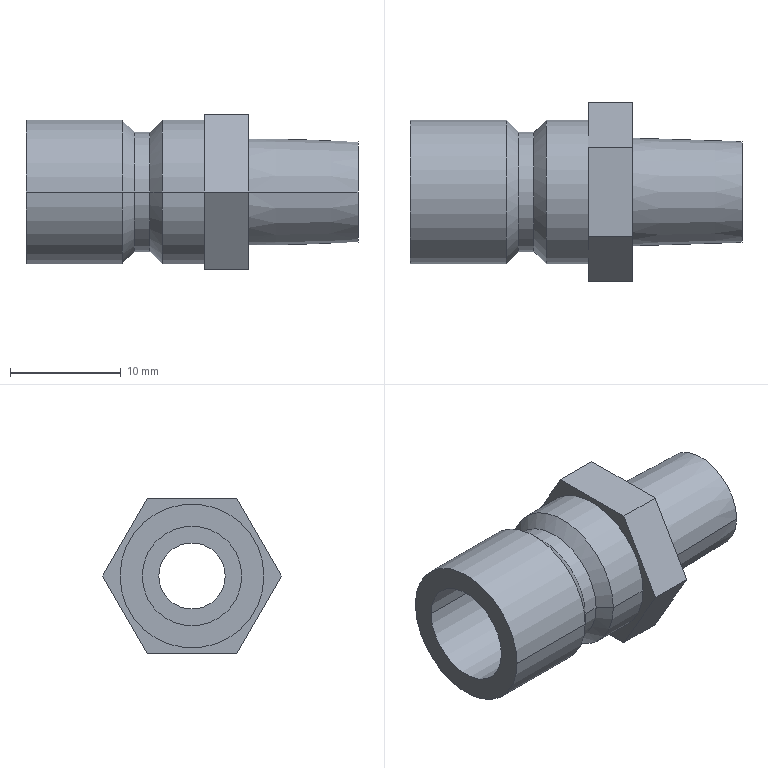Part | Creo | 1 solid | 27 faces | box 30 x 16.166 x 14 mm | volume 1882 mm3 | plane 11 | cylinder 10 | cone 6 | commonest cylinder face diameters 13 x4 6 x2 9 x2 10.8 x2
STEP:
#1=CARTESIAN_POINT('',(0.,0.,0.));
#2=DIRECTION('',(0.,0.,1.));
#3=DIRECTION('',(1.,0.,0.));
#4=AXIS2_PLACEMENT_3D('',#1,#2,#3);
#5=CARTESIAN_POINT('',(-220.1,-3.5,-74.09));
#6=VERTEX_POINT('',#5);
#7=CARTESIAN_POINT('',(-220.1,-16.5,-74.09));
#8=VERTEX_POINT('',#7);
#9=CARTESIAN_POINT('',(-220.1,-10.,-74.09));
#10=DIRECTION('',(-1.,0.,0.));
#11=DIRECTION('',(0.,1.,0.));
#12=AXIS2_PLACEMENT_3D('',#9,#10,#11);
#13=CIRCLE('',#12,6.5);
#14=EDGE_CURVE('',#6,#8,#13,.T.);
#15=ORIENTED_EDGE('',*,*,#14,.F.);
#16=CARTESIAN_POINT('',(-220.1,-10.,-74.09));
#17=DIRECTION('',(-1.,0.,0.));
#18=DIRECTION('',(0.,-1.,0.));
#19=AXIS2_PLACEMENT_3D('',#16,#17,#18);
#20=CIRCLE('',#19,6.5);
#21=EDGE_CURVE('',#8,#6,#20,.T.);
#22=ORIENTED_EDGE('',*,*,#21,.F.);
#23=EDGE_LOOP('',(#15,#22));
#24=FACE_OUTER_BOUND('',#23,.F.);
#25=CARTESIAN_POINT('',(-220.1,-5.5,-74.09));
#26=VERTEX_POINT('',#25);
#27=CARTESIAN_POINT('',(-220.1,-14.5,-74.09));
#28=VERTEX_POINT('',#27);
#29=CARTESIAN_POINT('',(-220.1,-10.,-74.09));
#30=DIRECTION('',(1.,0.,0.));
#31=DIRECTION('',(0.,1.,0.));
#32=AXIS2_PLACEMENT_3D('',#29,#30,#31);
#33=CIRCLE('',#32,4.5);
#34=EDGE_CURVE('',#26,#28,#33,.T.);
#35=ORIENTED_EDGE('',*,*,#34,.F.);
#36=CARTESIAN_POINT('',(-220.1,-10.,-74.09));
#37=DIRECTION('',(1.,0.,0.));
#38=DIRECTION('',(0.,-1.,0.));
#39=AXIS2_PLACEMENT_3D('',#36,#37,#38);
#40=CIRCLE('',#39,4.5);
#41=EDGE_CURVE('',#28,#26,#40,.T.);
#42=ORIENTED_EDGE('',*,*,#41,.F.);
#43=EDGE_LOOP('',(#35,#42));
#44=FACE_BOUND('',#43,.F.);
#45=CARTESIAN_POINT('',(-220.1,-10.,-67.59));
#46=DIRECTION('',(-1.,0.,0.));
#47=DIRECTION('',(0.,-1.,0.));
#48=AXIS2_PLACEMENT_3D('',#45,#46,#47);
#49=PLANE('',#48);
#50=ADVANCED_FACE('',(#24,#44),#49,.T.);
#51=ORIENTED_EDGE('',*,*,#14,.T.);
#52=CARTESIAN_POINT('',(-211.4,-16.5,-74.09));
#53=VERTEX_POINT('',#52);
#54=CARTESIAN_POINT('',(-220.1,-16.5,-74.09));
#55=DIRECTION('',(1.,0.,0.));
#56=VECTOR('',#55,8.7);
#57=LINE('',#54,#56);
#58=EDGE_CURVE('',#8,#53,#57,.T.);
#59=ORIENTED_EDGE('',*,*,#58,.T.);
#60=CARTESIAN_POINT('',(-211.4,-3.5,-74.09));
#61=VERTEX_POINT('',#60);
#62=CARTESIAN_POINT('',(-211.4,-10.,-74.09));
#63=DIRECTION('',(1.,0.,0.));
#64=DIRECTION('',(0.,-1.,0.));
#65=AXIS2_PLACEMENT_3D('',#62,#63,#64);
#66=CIRCLE('',#65,6.5);
#67=EDGE_CURVE('',#53,#61,#66,.T.);
#68=ORIENTED_EDGE('',*,*,#67,.T.);
#69=CARTESIAN_POINT('',(-220.1,-3.5,-74.09));
#70=DIRECTION('',(1.,0.,0.));
#71=VECTOR('',#70,8.7);
#72=LINE('',#69,#71);
#73=EDGE_CURVE('',#6,#61,#72,.T.);
#74=ORIENTED_EDGE('',*,*,#73,.F.);
#75=EDGE_LOOP('',(#51,#59,#68,#74));
#76=FACE_OUTER_BOUND('',#75,.F.);
#77=CARTESIAN_POINT('',(-200.,-10.,-74.09));
#78=DIRECTION('',(1.,0.,0.));
#79=DIRECTION('',(0.,1.,0.));
#80=AXIS2_PLACEMENT_3D('',#77,#78,#79);
#81=CYLINDRICAL_SURFACE('',#80,6.5);
#82=ADVANCED_FACE('',(#76),#81,.T.);
#83=ORIENTED_EDGE('',*,*,#21,.T.);
#84=ORIENTED_EDGE('',*,*,#73,.T.);
#85=CARTESIAN_POINT('',(-211.4,-10.,-74.09));
#86=DIRECTION('',(1.,0.,0.));
#87=DIRECTION('',(0.,1.,0.));
#88=AXIS2_PLACEMENT_3D('',#85,#86,#87);
#89=CIRCLE('',#88,6.5);
#90=EDGE_CURVE('',#61,#53,#89,.T.);
#91=ORIENTED_EDGE('',*,*,#90,.T.);
#92=ORIENTED_EDGE('',*,*,#58,.F.);
#93=EDGE_LOOP('',(#83,#84,#91,#92));
#94=FACE_OUTER_BOUND('',#93,.F.);
#95=CARTESIAN_POINT('',(-200.,-10.,-74.09));
#96=DIRECTION('',(1.,0.,0.));
#97=DIRECTION('',(0.,1.,0.));
#98=AXIS2_PLACEMENT_3D('',#95,#96,#97);
#99=CYLINDRICAL_SURFACE('',#98,6.5);
#100=ADVANCED_FACE('',(#94),#99,.T.);
#101=ORIENTED_EDGE('',*,*,#90,.F.);
#102=CARTESIAN_POINT('',(-210.3,-4.6,-74.09));
#103=VERTEX_POINT('',#102);
#104=CARTESIAN_POINT('',(-210.3,-4.6,-74.09));
#105=DIRECTION('',(-0.7071,0.7071,0.));
#106=VECTOR('',#105,1.556);
#107=LINE('',#104,#106);
#108=EDGE_CURVE('',#103,#61,#107,.T.);
#109=ORIENTED_EDGE('',*,*,#108,.F.);
#110=CARTESIAN_POINT('',(-210.3,-15.4,-74.09));
#111=VERTEX_POINT('',#110);
#112=CARTESIAN_POINT('',(-210.3,-10.,-74.09));
#113=DIRECTION('',(-1.,0.,0.));
#114=DIRECTION('',(0.,-1.,0.));
#115=AXIS2_PLACEMENT_3D('',#112,#113,#114);
#116=CIRCLE('',#115,5.4);
#117=EDGE_CURVE('',#111,#103,#116,.T.);
#118=ORIENTED_EDGE('',*,*,#117,.F.);
#119=CARTESIAN_POINT('',(-210.3,-15.4,-74.09));
#120=DIRECTION('',(-0.7071,-0.7071,0.));
#121=VECTOR('',#120,1.556);
#122=LINE('',#119,#121);
#123=EDGE_CURVE('',#111,#53,#122,.T.);
#124=ORIENTED_EDGE('',*,*,#123,.T.);
#125=EDGE_LOOP('',(#101,#109,#118,#124));
#126=FACE_OUTER_BOUND('',#125,.F.);
#127=CARTESIAN_POINT('',(-210.85,-10.,-74.09));
#128=DIRECTION('',(-1.,0.,0.));
#129=DIRECTION('',(0.,-1.,0.));
#130=AXIS2_PLACEMENT_3D('',#127,#128,#129);
#131=CONICAL_SURFACE('',#130,5.95,45.);
#132=ADVANCED_FACE('',(#126),#131,.T.);
#133=ORIENTED_EDGE('',*,*,#67,.F.);
#134=ORIENTED_EDGE('',*,*,#123,.F.);
#135=CARTESIAN_POINT('',(-210.3,-10.,-74.09));
#136=DIRECTION('',(-1.,0.,0.));
#137=DIRECTION('',(0.,1.,0.));
#138=AXIS2_PLACEMENT_3D('',#135,#136,#137);
#139=CIRCLE('',#138,5.4);
#140=EDGE_CURVE('',#103,#111,#139,.T.);
#141=ORIENTED_EDGE('',*,*,#140,.F.);
#142=ORIENTED_EDGE('',*,*,#108,.T.);
#143=EDGE_LOOP('',(#133,#134,#141,#142));
#144=FACE_OUTER_BOUND('',#143,.F.);
#145=CARTESIAN_POINT('',(-210.85,-10.,-74.09));
#146=DIRECTION('',(-1.,0.,0.));
#147=DIRECTION('',(0.,-1.,0.));
#148=AXIS2_PLACEMENT_3D('',#145,#146,#147);
#149=CONICAL_SURFACE('',#148,5.95,45.);
#150=ADVANCED_FACE('',(#144),#149,.T.);
#151=ORIENTED_EDGE('',*,*,#140,.T.);
#152=CARTESIAN_POINT('',(-208.9,-15.4,-74.09));
#153=VERTEX_POINT('',#152);
#154=CARTESIAN_POINT('',(-210.3,-15.4,-74.09));
#155=DIRECTION('',(1.,0.,0.));
#156=VECTOR('',#155,1.4);
#157=LINE('',#154,#156);
#158=EDGE_CURVE('',#111,#153,#157,.T.);
#159=ORIENTED_EDGE('',*,*,#158,.T.);
#160=CARTESIAN_POINT('',(-208.9,-4.6,-74.09));
#161=VERTEX_POINT('',#160);
#162=CARTESIAN_POINT('',(-208.9,-10.,-74.09));
#163=DIRECTION('',(1.,0.,0.));
#164=DIRECTION('',(0.,-1.,0.));
#165=AXIS2_PLACEMENT_3D('',#162,#163,#164);
#166=CIRCLE('',#165,5.4);
#167=EDGE_CURVE('',#153,#161,#166,.T.);
#168=ORIENTED_EDGE('',*,*,#167,.T.);
#169=CARTESIAN_POINT('',(-210.3,-4.6,-74.09));
#170=DIRECTION('',(1.,0.,0.));
#171=VECTOR('',#170,1.4);
#172=LINE('',#169,#171);
#173=EDGE_CURVE('',#103,#161,#172,.T.);
#174=ORIENTED_EDGE('',*,*,#173,.F.);
#175=EDGE_LOOP('',(#151,#159,#168,#174));
#176=FACE_OUTER_BOUND('',#175,.F.);
#177=CARTESIAN_POINT('',(-200.,-10.,-74.09));
#178=DIRECTION('',(1.,0.,0.));
#179=DIRECTION('',(0.,1.,0.));
#180=AXIS2_PLACEMENT_3D('',#177,#178,#179);
#181=CYLINDRICAL_SURFACE('',#180,5.4);
#182=ADVANCED_FACE('',(#176),#181,.T.);
#183=ORIENTED_EDGE('',*,*,#117,.T.);
#184=ORIENTED_EDGE('',*,*,#173,.T.);
#185=CARTESIAN_POINT('',(-208.9,-10.,-74.09));
#186=DIRECTION('',(1.,0.,0.));
#187=DIRECTION('',(0.,1.,0.));
#188=AXIS2_PLACEMENT_3D('',#185,#186,#187);
#189=CIRCLE('',#188,5.4);
#190=EDGE_CURVE('',#161,#153,#189,.T.);
#191=ORIENTED_EDGE('',*,*,#190,.T.);
#192=ORIENTED_EDGE('',*,*,#158,.F.);
#193=EDGE_LOOP('',(#183,#184,#191,#192));
#194=FACE_OUTER_BOUND('',#193,.F.);
#195=CARTESIAN_POINT('',(-200.,-10.,-74.09));
#196=DIRECTION('',(1.,0.,0.));
#197=DIRECTION('',(0.,1.,0.));
#198=AXIS2_PLACEMENT_3D('',#195,#196,#197);
#199=CYLINDRICAL_SURFACE('',#198,5.4);
#200=ADVANCED_FACE('',(#194),#199,.T.);
#201=ORIENTED_EDGE('',*,*,#190,.F.);
#202=CARTESIAN_POINT('',(-207.8,-3.5,-74.09));
#203=VERTEX_POINT('',#202);
#204=CARTESIAN_POINT('',(-208.9,-4.6,-74.09));
#205=DIRECTION('',(0.7071,0.7071,0.));
#206=VECTOR('',#205,1.556);
#207=LINE('',#204,#206);
#208=EDGE_CURVE('',#161,#203,#207,.T.);
#209=ORIENTED_EDGE('',*,*,#208,.T.);
#210=CARTESIAN_POINT('',(-207.8,-16.5,-74.09));
#211=VERTEX_POINT('',#210);
#212=CARTESIAN_POINT('',(-207.8,-10.,-74.09));
#213=DIRECTION('',(-1.,0.,0.));
#214=DIRECTION('',(0.,-1.,0.));
#215=AXIS2_PLACEMENT_3D('',#212,#213,#214);
#216=CIRCLE('',#215,6.5);
#217=EDGE_CURVE('',#211,#203,#216,.T.);
#218=ORIENTED_EDGE('',*,*,#217,.F.);
#219=CARTESIAN_POINT('',(-208.9,-15.4,-74.09));
#220=DIRECTION('',(0.7071,-0.7071,0.));
#221=VECTOR('',#220,1.556);
#222=LINE('',#219,#221);
#223=EDGE_CURVE('',#153,#211,#222,.T.);
#224=ORIENTED_EDGE('',*,*,#223,.F.);
#225=EDGE_LOOP('',(#201,#209,#218,#224));
#226=FACE_OUTER_BOUND('',#225,.F.);
#227=CARTESIAN_POINT('',(-208.35,-10.,-74.09));
#228=DIRECTION('',(1.,0.,0.));
#229=DIRECTION('',(0.,1.,0.));
#230=AXIS2_PLACEMENT_3D('',#227,#228,#229);
#231=CONICAL_SURFACE('',#230,5.95,45.);
#232=ADVANCED_FACE('',(#226),#231,.T.);
#233=ORIENTED_EDGE('',*,*,#167,.F.);
#234=ORIENTED_EDGE('',*,*,#223,.T.);
#235=CARTESIAN_POINT('',(-207.8,-10.,-74.09));
#236=DIRECTION('',(-1.,0.,0.));
#237=DIRECTION('',(0.,1.,0.));
#238=AXIS2_PLACEMENT_3D('',#235,#236,#237);
#239=CIRCLE('',#238,6.5);
#240=EDGE_CURVE('',#203,#211,#239,.T.);
#241=ORIENTED_EDGE('',*,*,#240,.F.);
#242=ORIENTED_EDGE('',*,*,#208,.F.);
#243=EDGE_LOOP('',(#233,#234,#241,#242));
#244=FACE_OUTER_BOUND('',#243,.F.);
#245=CARTESIAN_POINT('',(-208.35,-10.,-74.09));
#246=DIRECTION('',(1.,0.,0.));
#247=DIRECTION('',(0.,1.,0.));
#248=AXIS2_PLACEMENT_3D('',#245,#246,#247);
#249=CONICAL_SURFACE('',#248,5.95,45.);
#250=ADVANCED_FACE('',(#244),#249,.T.);
#251=ORIENTED_EDGE('',*,*,#240,.T.);
#252=CARTESIAN_POINT('',(-204.,-16.5,-74.09));
#253=VERTEX_POINT('',#252);
#254=CARTESIAN_POINT('',(-207.8,-16.5,-74.09));
#255=DIRECTION('',(1.,0.,0.));
#256=VECTOR('',#255,3.8);
#257=LINE('',#254,#256);
#258=EDGE_CURVE('',#211,#253,#257,.T.);
#259=ORIENTED_EDGE('',*,*,#258,.T.);
#260=CARTESIAN_POINT('',(-204.,-3.5,-74.09));
#261=VERTEX_POINT('',#260);
#262=CARTESIAN_POINT('',(-204.,-10.,-74.09));
#263=DIRECTION('',(1.,0.,0.));
#264=DIRECTION('',(0.,-1.,0.));
#265=AXIS2_PLACEMENT_3D('',#262,#263,#264);
#266=CIRCLE('',#265,6.5);
#267=EDGE_CURVE('',#253,#261,#266,.T.);
#268=ORIENTED_EDGE('',*,*,#267,.T.);
#269=CARTESIAN_POINT('',(-207.8,-3.5,-74.09));
#270=DIRECTION('',(1.,0.,0.));
#271=VECTOR('',#270,3.8);
#272=LINE('',#269,#271);
#273=EDGE_CURVE('',#203,#261,#272,.T.);
#274=ORIENTED_EDGE('',*,*,#273,.F.);
#275=EDGE_LOOP('',(#251,#259,#268,#274));
#276=FACE_OUTER_BOUND('',#275,.F.);
#277=CARTESIAN_POINT('',(-200.,-10.,-74.09));
#278=DIRECTION('',(1.,0.,0.));
#279=DIRECTION('',(0.,1.,0.));
#280=AXIS2_PLACEMENT_3D('',#277,#278,#279);
#281=CYLINDRICAL_SURFACE('',#280,6.5);
#282=ADVANCED_FACE('',(#276),#281,.T.);
#283=ORIENTED_EDGE('',*,*,#217,.T.);
#284=ORIENTED_EDGE('',*,*,#273,.T.);
#285=CARTESIAN_POINT('',(-204.,-10.,-74.09));
#286=DIRECTION('',(1.,0.,0.));
#287=DIRECTION('',(0.,1.,0.));
#288=AXIS2_PLACEMENT_3D('',#285,#286,#287);
#289=CIRCLE('',#288,6.5);
#290=EDGE_CURVE('',#261,#253,#289,.T.);
#291=ORIENTED_EDGE('',*,*,#290,.T.);
#292=ORIENTED_EDGE('',*,*,#258,.F.);
#293=EDGE_LOOP('',(#283,#284,#291,#292));
#294=FACE_OUTER_BOUND('',#293,.F.);
#295=CARTESIAN_POINT('',(-200.,-10.,-74.09));
#296=DIRECTION('',(1.,0.,0.));
#297=DIRECTION('',(0.,1.,0.));
#298=AXIS2_PLACEMENT_3D('',#295,#296,#297);
#299=CYLINDRICAL_SURFACE('',#298,6.5);
#300=ADVANCED_FACE('',(#294),#299,.T.);
#301=CARTESIAN_POINT('',(-204.,-18.083,-74.09));
#302=VERTEX_POINT('',#301);
#303=CARTESIAN_POINT('',(-204.,-14.041,-67.09));
#304=VERTEX_POINT('',#303);
#305=CARTESIAN_POINT('',(-204.,-18.083,-74.09));
#306=DIRECTION('',(0.,0.5,0.866));
#307=VECTOR('',#306,8.083);
#308=LINE('',#305,#307);
#309=EDGE_CURVE('',#302,#304,#308,.T.);
#310=ORIENTED_EDGE('',*,*,#309,.F.);
#311=CARTESIAN_POINT('',(-204.,-14.041,-81.09));
#312=VERTEX_POINT('',#311);
#313=CARTESIAN_POINT('',(-204.,-14.041,-81.09));
#314=DIRECTION('',(0.,-0.5,0.866));
#315=VECTOR('',#314,8.083);
#316=LINE('',#313,#315);
#317=EDGE_CURVE('',#312,#302,#316,.T.);
#318=ORIENTED_EDGE('',*,*,#317,.F.);
#319=CARTESIAN_POINT('',(-204.,-5.959,-81.09));
#320=VERTEX_POINT('',#319);
#321=CARTESIAN_POINT('',(-204.,-5.959,-81.09));
#322=DIRECTION('',(0.,-1.,0.));
#323=VECTOR('',#322,8.083);
#324=LINE('',#321,#323);
#325=EDGE_CURVE('',#320,#312,#324,.T.);
#326=ORIENTED_EDGE('',*,*,#325,.F.);
#327=CARTESIAN_POINT('',(-204.,-1.917,-74.09));
#328=VERTEX_POINT('',#327);
#329=CARTESIAN_POINT('',(-204.,-1.917,-74.09));
#330=DIRECTION('',(0.,-0.5,-0.866));
#331=VECTOR('',#330,8.083);
#332=LINE('',#329,#331);
#333=EDGE_CURVE('',#328,#320,#332,.T.);
#334=ORIENTED_EDGE('',*,*,#333,.F.);
#335=CARTESIAN_POINT('',(-204.,-5.959,-67.09));
#336=VERTEX_POINT('',#335);
#337=CARTESIAN_POINT('',(-204.,-5.959,-67.09));
#338=DIRECTION('',(0.,0.5,-0.866));
#339=VECTOR('',#338,8.083);
#340=LINE('',#337,#339);
#341=EDGE_CURVE('',#336,#328,#340,.T.);
#342=ORIENTED_EDGE('',*,*,#341,.F.);
#343=CARTESIAN_POINT('',(-204.,-14.041,-67.09));
#344=DIRECTION('',(0.,1.,0.));
#345=VECTOR('',#344,8.083);
#346=LINE('',#343,#345);
#347=EDGE_CURVE('',#304,#336,#346,.T.);
#348=ORIENTED_EDGE('',*,*,#347,.F.);
#349=EDGE_LOOP('',(#310,#318,#326,#334,#342,#348));
#350=FACE_OUTER_BOUND('',#349,.F.);
#351=ORIENTED_EDGE('',*,*,#290,.F.);
#352=ORIENTED_EDGE('',*,*,#267,.F.);
#353=EDGE_LOOP('',(#351,#352));
#354=FACE_BOUND('',#353,.F.);
#355=CARTESIAN_POINT('',(-204.,-10.,-67.09));
#356=DIRECTION('',(-1.,0.,0.));
#357=DIRECTION('',(0.,-1.,0.));
#358=AXIS2_PLACEMENT_3D('',#355,#356,#357);
#359=PLANE('',#358);
#360=ADVANCED_FACE('',(#350,#354),#359,.T.);
#361=ORIENTED_EDGE('',*,*,#309,.T.);
#362=CARTESIAN_POINT('',(-200.,-14.041,-67.09));
#363=VERTEX_POINT('',#362);
#364=CARTESIAN_POINT('',(-200.,-14.041,-67.09));
#365=DIRECTION('',(-1.,0.,0.));
#366=VECTOR('',#365,4.);
#367=LINE('',#364,#366);
#368=EDGE_CURVE('',#363,#304,#367,.T.);
#369=ORIENTED_EDGE('',*,*,#368,.F.);
#370=CARTESIAN_POINT('',(-200.,-18.083,-74.09));
#371=VERTEX_POINT('',#370);
#372=CARTESIAN_POINT('',(-200.,-14.041,-67.09));
#373=DIRECTION('',(0.,-0.5,-0.866));
#374=VECTOR('',#373,8.083);
#375=LINE('',#372,#374);
#376=EDGE_CURVE('',#363,#371,#375,.T.);
#377=ORIENTED_EDGE('',*,*,#376,.T.);
#378=CARTESIAN_POINT('',(-200.,-18.083,-74.09));
#379=DIRECTION('',(-1.,0.,0.));
#380=VECTOR('',#379,4.);
#381=LINE('',#378,#380);
#382=EDGE_CURVE('',#371,#302,#381,.T.);
#383=ORIENTED_EDGE('',*,*,#382,.T.);
#384=EDGE_LOOP('',(#361,#369,#377,#383));
#385=FACE_OUTER_BOUND('',#384,.F.);
#386=CARTESIAN_POINT('',(-204.,-14.041,-67.09));
#387=DIRECTION('',(0.,-0.866,0.5));
#388=DIRECTION('',(0.,0.5,0.866));
#389=AXIS2_PLACEMENT_3D('',#386,#387,#388);
#390=PLANE('',#389);
#391=ADVANCED_FACE('',(#385),#390,.T.);
#392=ORIENTED_EDGE('',*,*,#347,.T.);
#393=CARTESIAN_POINT('',(-200.,-5.959,-67.09));
#394=VERTEX_POINT('',#393);
#395=CARTESIAN_POINT('',(-200.,-5.959,-67.09));
#396=DIRECTION('',(-1.,0.,0.));
#397=VECTOR('',#396,4.);
#398=LINE('',#395,#397);
#399=EDGE_CURVE('',#394,#336,#398,.T.);
#400=ORIENTED_EDGE('',*,*,#399,.F.);
#401=CARTESIAN_POINT('',(-200.,-14.041,-67.09));
#402=DIRECTION('',(0.,1.,0.));
#403=VECTOR('',#402,8.083);
#404=LINE('',#401,#403);
#405=EDGE_CURVE('',#363,#394,#404,.T.);
#406=ORIENTED_EDGE('',*,*,#405,.F.);
#407=ORIENTED_EDGE('',*,*,#368,.T.);
#408=EDGE_LOOP('',(#392,#400,#406,#407));
#409=FACE_OUTER_BOUND('',#408,.F.);
#410=CARTESIAN_POINT('',(-204.,-5.959,-67.09));
#411=DIRECTION('',(0.,0.,1.));
#412=DIRECTION('',(0.,1.,0.));
#413=AXIS2_PLACEMENT_3D('',#410,#411,#412);
#414=PLANE('',#413);
#415=ADVANCED_FACE('',(#409),#414,.T.);
#416=ORIENTED_EDGE('',*,*,#341,.T.);
#417=CARTESIAN_POINT('',(-200.,-1.917,-74.09));
#418=VERTEX_POINT('',#417);
#419=CARTESIAN_POINT('',(-200.,-1.917,-74.09));
#420=DIRECTION('',(-1.,0.,0.));
#421=VECTOR('',#420,4.);
#422=LINE('',#419,#421);
#423=EDGE_CURVE('',#418,#328,#422,.T.);
#424=ORIENTED_EDGE('',*,*,#423,.F.);
#425=CARTESIAN_POINT('',(-200.,-1.917,-74.09));
#426=DIRECTION('',(0.,-0.5,0.866));
#427=VECTOR('',#426,8.083);
#428=LINE('',#425,#427);
#429=EDGE_CURVE('',#418,#394,#428,.T.);
#430=ORIENTED_EDGE('',*,*,#429,.T.);
#431=ORIENTED_EDGE('',*,*,#399,.T.);
#432=EDGE_LOOP('',(#416,#424,#430,#431));
#433=FACE_OUTER_BOUND('',#432,.F.);
#434=CARTESIAN_POINT('',(-204.,-1.917,-74.09));
#435=DIRECTION('',(0.,0.866,0.5));
#436=DIRECTION('',(0.,0.5,-0.866));
#437=AXIS2_PLACEMENT_3D('',#434,#435,#436);
#438=PLANE('',#437);
#439=ADVANCED_FACE('',(#433),#438,.T.);
#440=ORIENTED_EDGE('',*,*,#333,.T.);
#441=CARTESIAN_POINT('',(-200.,-5.959,-81.09));
#442=VERTEX_POINT('',#441);
#443=CARTESIAN_POINT('',(-200.,-5.959,-81.09));
#444=DIRECTION('',(-1.,0.,0.));
#445=VECTOR('',#444,4.);
#446=LINE('',#443,#445);
#447=EDGE_CURVE('',#442,#320,#446,.T.);
#448=ORIENTED_EDGE('',*,*,#447,.F.);
#449=CARTESIAN_POINT('',(-200.,-5.959,-81.09));
#450=DIRECTION('',(0.,0.5,0.866));
#451=VECTOR('',#450,8.083);
#452=LINE('',#449,#451);
#453=EDGE_CURVE('',#442,#418,#452,.T.);
#454=ORIENTED_EDGE('',*,*,#453,.T.);
#455=ORIENTED_EDGE('',*,*,#423,.T.);
#456=EDGE_LOOP('',(#440,#448,#454,#455));
#457=FACE_OUTER_BOUND('',#456,.F.);
#458=CARTESIAN_POINT('',(-204.,-5.959,-81.09));
#459=DIRECTION('',(0.,0.866,-0.5));
#460=DIRECTION('',(0.,-0.5,-0.866));
#461=AXIS2_PLACEMENT_3D('',#458,#459,#460);
#462=PLANE('',#461);
#463=ADVANCED_FACE('',(#457),#462,.T.);
#464=ORIENTED_EDGE('',*,*,#325,.T.);
#465=CARTESIAN_POINT('',(-200.,-14.041,-81.09));
#466=VERTEX_POINT('',#465);
#467=CARTESIAN_POINT('',(-200.,-14.041,-81.09));
#468=DIRECTION('',(-1.,0.,0.));
#469=VECTOR('',#468,4.);
#470=LINE('',#467,#469);
#471=EDGE_CURVE('',#466,#312,#470,.T.);
#472=ORIENTED_EDGE('',*,*,#471,.F.);
#473=CARTESIAN_POINT('',(-200.,-5.959,-81.09));
#474=DIRECTION('',(0.,-1.,0.));
#475=VECTOR('',#474,8.083);
#476=LINE('',#473,#475);
#477=EDGE_CURVE('',#442,#466,#476,.T.);
#478=ORIENTED_EDGE('',*,*,#477,.F.);
#479=ORIENTED_EDGE('',*,*,#447,.T.);
#480=EDGE_LOOP('',(#464,#472,#478,#479));
#481=FACE_OUTER_BOUND('',#480,.F.);
#482=CARTESIAN_POINT('',(-204.,-14.041,-81.09));
#483=DIRECTION('',(0.,0.,-1.));
#484=DIRECTION('',(0.,-1.,0.));
#485=AXIS2_PLACEMENT_3D('',#482,#483,#484);
#486=PLANE('',#485);
#487=ADVANCED_FACE('',(#481),#486,.T.);
#488=ORIENTED_EDGE('',*,*,#317,.T.);
#489=ORIENTED_EDGE('',*,*,#382,.F.);
#490=CARTESIAN_POINT('',(-200.,-18.083,-74.09));
#491=DIRECTION('',(0.,0.5,-0.866));
#492=VECTOR('',#491,8.083);
#493=LINE('',#490,#492);
#494=EDGE_CURVE('',#371,#466,#493,.T.);
#495=ORIENTED_EDGE('',*,*,#494,.T.);
#496=ORIENTED_EDGE('',*,*,#471,.T.);
#497=EDGE_LOOP('',(#488,#489,#495,#496));
#498=FACE_OUTER_BOUND('',#497,.F.);
#499=CARTESIAN_POINT('',(-204.,-18.083,-74.09));
#500=DIRECTION('',(0.,-0.866,-0.5));
#501=DIRECTION('',(0.,-0.5,0.866));
#502=AXIS2_PLACEMENT_3D('',#499,#500,#501);
#503=PLANE('',#502);
#504=ADVANCED_FACE('',(#498),#503,.T.);
#505=ORIENTED_EDGE('',*,*,#453,.F.);
#506=ORIENTED_EDGE('',*,*,#477,.T.);
#507=ORIENTED_EDGE('',*,*,#494,.F.);
#508=ORIENTED_EDGE('',*,*,#376,.F.);
#509=ORIENTED_EDGE('',*,*,#405,.T.);
#510=ORIENTED_EDGE('',*,*,#429,.F.);
#511=EDGE_LOOP('',(#505,#506,#507,#508,#509,#510));
#512=FACE_OUTER_BOUND('',#511,.F.);
#513=CARTESIAN_POINT('',(-200.,-5.135,-74.09));
#514=VERTEX_POINT('',#513);
#515=CARTESIAN_POINT('',(-200.,-14.865,-74.09));
#516=VERTEX_POINT('',#515);
#517=CARTESIAN_POINT('',(-200.,-10.,-74.09));
#518=DIRECTION('',(-1.,0.,0.));
#519=DIRECTION('',(0.,1.,0.));
#520=AXIS2_PLACEMENT_3D('',#517,#518,#519);
#521=CIRCLE('',#520,4.865);
#522=EDGE_CURVE('',#514,#516,#521,.T.);
#523=ORIENTED_EDGE('',*,*,#522,.F.);
#524=CARTESIAN_POINT('',(-200.,-10.,-74.09));
#525=DIRECTION('',(-1.,0.,0.));
#526=DIRECTION('',(0.,-1.,0.));
#527=AXIS2_PLACEMENT_3D('',#524,#525,#526);
#528=CIRCLE('',#527,4.865);
#529=EDGE_CURVE('',#516,#514,#528,.T.);
#530=ORIENTED_EDGE('',*,*,#529,.F.);
#531=EDGE_LOOP('',(#523,#530));
#532=FACE_BOUND('',#531,.F.);
#533=CARTESIAN_POINT('',(-200.,-10.,-69.225));
#534=DIRECTION('',(1.,0.,0.));
#535=DIRECTION('',(0.,1.,0.));
#536=AXIS2_PLACEMENT_3D('',#533,#534,#535);
#537=PLANE('',#536);
#538=ADVANCED_FACE('',(#512,#532),#537,.T.);
#539=ORIENTED_EDGE('',*,*,#522,.T.);
#540=CARTESIAN_POINT('',(-190.1,-14.554,-74.09));
#541=VERTEX_POINT('',#540);
#542=CARTESIAN_POINT('',(-190.1,-14.554,-74.09));
#543=DIRECTION('',(-0.9995,-0.03141,0.));
#544=VECTOR('',#543,9.905);
#545=LINE('',#542,#544);
#546=EDGE_CURVE('',#541,#516,#545,.T.);
#547=ORIENTED_EDGE('',*,*,#546,.F.);
#548=CARTESIAN_POINT('',(-190.1,-5.446,-74.09));
#549=VERTEX_POINT('',#548);
#550=CARTESIAN_POINT('',(-190.1,-10.,-74.09));
#551=DIRECTION('',(1.,0.,0.));
#552=DIRECTION('',(0.,-1.,0.));
#553=AXIS2_PLACEMENT_3D('',#550,#551,#552);
#554=CIRCLE('',#553,4.554);
#555=EDGE_CURVE('',#541,#549,#554,.T.);
#556=ORIENTED_EDGE('',*,*,#555,.T.);
#557=CARTESIAN_POINT('',(-190.1,-5.446,-74.09));
#558=DIRECTION('',(-0.9995,0.03141,0.));
#559=VECTOR('',#558,9.905);
#560=LINE('',#557,#559);
#561=EDGE_CURVE('',#549,#514,#560,.T.);
#562=ORIENTED_EDGE('',*,*,#561,.T.);
#563=EDGE_LOOP('',(#539,#547,#556,#562));
#564=FACE_OUTER_BOUND('',#563,.F.);
#565=CARTESIAN_POINT('',(-195.05,-10.,-74.09));
#566=DIRECTION('',(-1.,0.,0.));
#567=DIRECTION('',(0.,-1.,0.));
#568=AXIS2_PLACEMENT_3D('',#565,#566,#567);
#569=CONICAL_SURFACE('',#568,4.709,1.8);
#570=ADVANCED_FACE('',(#564),#569,.T.);
#571=ORIENTED_EDGE('',*,*,#529,.T.);
#572=ORIENTED_EDGE('',*,*,#561,.F.);
#573=CARTESIAN_POINT('',(-190.1,-10.,-74.09));
#574=DIRECTION('',(1.,0.,0.));
#575=DIRECTION('',(0.,1.,0.));
#576=AXIS2_PLACEMENT_3D('',#573,#574,#575);
#577=CIRCLE('',#576,4.554);
#578=EDGE_CURVE('',#549,#541,#577,.T.);
#579=ORIENTED_EDGE('',*,*,#578,.T.);
#580=ORIENTED_EDGE('',*,*,#546,.T.);
#581=EDGE_LOOP('',(#571,#572,#579,#580));
#582=FACE_OUTER_BOUND('',#581,.F.);
#583=CARTESIAN_POINT('',(-195.05,-10.,-74.09));
#584=DIRECTION('',(-1.,0.,0.));
#585=DIRECTION('',(0.,-1.,0.));
#586=AXIS2_PLACEMENT_3D('',#583,#584,#585);
#587=CONICAL_SURFACE('',#586,4.709,1.8);
#588=ADVANCED_FACE('',(#582),#587,.T.);
#589=ORIENTED_EDGE('',*,*,#578,.F.);
#590=ORIENTED_EDGE('',*,*,#555,.F.);
#591=EDGE_LOOP('',(#589,#590));
#592=FACE_OUTER_BOUND('',#591,.F.);
#593=CARTESIAN_POINT('',(-190.1,-7.,-74.09));
#594=VERTEX_POINT('',#593);
#595=CARTESIAN_POINT('',(-190.1,-13.,-74.09));
#596=VERTEX_POINT('',#595);
#597=CARTESIAN_POINT('',(-190.1,-10.,-74.09));
#598=DIRECTION('',(-1.,0.,0.));
#599=DIRECTION('',(0.,1.,0.));
#600=AXIS2_PLACEMENT_3D('',#597,#598,#599);
#601=CIRCLE('',#600,3.);
#602=EDGE_CURVE('',#594,#596,#601,.T.);
#603=ORIENTED_EDGE('',*,*,#602,.F.);
#604=CARTESIAN_POINT('',(-190.1,-10.,-74.09));
#605=DIRECTION('',(-1.,0.,0.));
#606=DIRECTION('',(0.,-1.,0.));
#607=AXIS2_PLACEMENT_3D('',#604,#605,#606);
#608=CIRCLE('',#607,3.);
#609=EDGE_CURVE('',#596,#594,#608,.T.);
#610=ORIENTED_EDGE('',*,*,#609,.F.);
#611=EDGE_LOOP('',(#603,#610));
#612=FACE_BOUND('',#611,.F.);
#613=CARTESIAN_POINT('',(-190.1,-10.,-74.09));
#614=DIRECTION('',(1.,0.,0.));
#615=DIRECTION('',(0.,1.,0.));
#616=AXIS2_PLACEMENT_3D('',#613,#614,#615);
#617=PLANE('',#616);
#618=ADVANCED_FACE('',(#592,#612),#617,.T.);
#619=ORIENTED_EDGE('',*,*,#602,.T.);
#620=CARTESIAN_POINT('',(-201.1,-13.,-74.09));
#621=VERTEX_POINT('',#620);
#622=CARTESIAN_POINT('',(-201.1,-13.,-74.09));
#623=DIRECTION('',(1.,0.,0.));
#624=VECTOR('',#623,11.);
#625=LINE('',#622,#624);
#626=EDGE_CURVE('',#621,#596,#625,.T.);
#627=ORIENTED_EDGE('',*,*,#626,.F.);
#628=CARTESIAN_POINT('',(-201.1,-7.,-74.09));
#629=VERTEX_POINT('',#628);
#630=CARTESIAN_POINT('',(-201.1,-10.,-74.09));
#631=DIRECTION('',(1.,0.,0.));
#632=DIRECTION('',(0.,-1.,0.));
#633=AXIS2_PLACEMENT_3D('',#630,#631,#632);
#634=CIRCLE('',#633,3.);
#635=EDGE_CURVE('',#621,#629,#634,.T.);
#636=ORIENTED_EDGE('',*,*,#635,.T.);
#637=CARTESIAN_POINT('',(-201.1,-7.,-74.09));
#638=DIRECTION('',(1.,0.,0.));
#639=VECTOR('',#638,11.);
#640=LINE('',#637,#639);
#641=EDGE_CURVE('',#629,#594,#640,.T.);
#642=ORIENTED_EDGE('',*,*,#641,.T.);
#643=EDGE_LOOP('',(#619,#627,#636,#642));
#644=FACE_OUTER_BOUND('',#643,.F.);
#645=CARTESIAN_POINT('',(-200.,-10.,-74.09));
#646=DIRECTION('',(1.,0.,0.));
#647=DIRECTION('',(0.,1.,0.));
#648=AXIS2_PLACEMENT_3D('',#645,#646,#647);
#649=CYLINDRICAL_SURFACE('',#648,3.);
#650=ADVANCED_FACE('',(#644),#649,.F.);
#651=ORIENTED_EDGE('',*,*,#609,.T.);
#652=ORIENTED_EDGE('',*,*,#641,.F.);
#653=CARTESIAN_POINT('',(-201.1,-10.,-74.09));
#654=DIRECTION('',(1.,0.,0.));
#655=DIRECTION('',(0.,1.,0.));
#656=AXIS2_PLACEMENT_3D('',#653,#654,#655);
#657=CIRCLE('',#656,3.);
#658=EDGE_CURVE('',#629,#621,#657,.T.);
#659=ORIENTED_EDGE('',*,*,#658,.T.);
#660=ORIENTED_EDGE('',*,*,#626,.T.);
#661=EDGE_LOOP('',(#651,#652,#659,#660));
#662=FACE_OUTER_BOUND('',#661,.F.);
#663=CARTESIAN_POINT('',(-200.,-10.,-74.09));
#664=DIRECTION('',(1.,0.,0.));
#665=DIRECTION('',(0.,1.,0.));
#666=AXIS2_PLACEMENT_3D('',#663,#664,#665);
#667=CYLINDRICAL_SURFACE('',#666,3.);
#668=ADVANCED_FACE('',(#662),#667,.F.);
#669=CARTESIAN_POINT('',(-201.1,-5.5,-74.09));
#670=VERTEX_POINT('',#669);
#671=CARTESIAN_POINT('',(-201.1,-14.5,-74.09));
#672=VERTEX_POINT('',#671);
#673=CARTESIAN_POINT('',(-201.1,-10.,-74.09));
#674=DIRECTION('',(-1.,0.,0.));
#675=DIRECTION('',(0.,1.,0.));
#676=AXIS2_PLACEMENT_3D('',#673,#674,#675);
#677=CIRCLE('',#676,4.5);
#678=EDGE_CURVE('',#670,#672,#677,.T.);
#679=ORIENTED_EDGE('',*,*,#678,.F.);
#680=CARTESIAN_POINT('',(-201.1,-10.,-74.09));
#681=DIRECTION('',(-1.,0.,0.));
#682=DIRECTION('',(0.,-1.,0.));
#683=AXIS2_PLACEMENT_3D('',#680,#681,#682);
#684=CIRCLE('',#683,4.5);
#685=EDGE_CURVE('',#672,#670,#684,.T.);
#686=ORIENTED_EDGE('',*,*,#685,.F.);
#687=EDGE_LOOP('',(#679,#686));
#688=FACE_OUTER_BOUND('',#687,.F.);
#689=ORIENTED_EDGE('',*,*,#658,.F.);
#690=ORIENTED_EDGE('',*,*,#635,.F.);
#691=EDGE_LOOP('',(#689,#690));
#692=FACE_BOUND('',#691,.F.);
#693=CARTESIAN_POINT('',(-201.1,-14.5,-74.09));
#694=DIRECTION('',(-1.,0.,0.));
#695=DIRECTION('',(0.,-1.,0.));
#696=AXIS2_PLACEMENT_3D('',#693,#694,#695);
#697=PLANE('',#696);
#698=ADVANCED_FACE('',(#688,#692),#697,.T.);
#699=ORIENTED_EDGE('',*,*,#678,.T.);
#700=CARTESIAN_POINT('',(-220.1,-14.5,-74.09));
#701=DIRECTION('',(1.,0.,0.));
#702=VECTOR('',#701,19.);
#703=LINE('',#700,#702);
#704=EDGE_CURVE('',#28,#672,#703,.T.);
#705=ORIENTED_EDGE('',*,*,#704,.F.);
#706=ORIENTED_EDGE('',*,*,#41,.T.);
#707=CARTESIAN_POINT('',(-220.1,-5.5,-74.09));
#708=DIRECTION('',(1.,0.,0.));
#709=VECTOR('',#708,19.);
#710=LINE('',#707,#709);
#711=EDGE_CURVE('',#26,#670,#710,.T.);
#712=ORIENTED_EDGE('',*,*,#711,.T.);
#713=EDGE_LOOP('',(#699,#705,#706,#712));
#714=FACE_OUTER_BOUND('',#713,.F.);
#715=CARTESIAN_POINT('',(-200.,-10.,-74.09));
#716=DIRECTION('',(1.,0.,0.));
#717=DIRECTION('',(0.,1.,0.));
#718=AXIS2_PLACEMENT_3D('',#715,#716,#717);
#719=CYLINDRICAL_SURFACE('',#718,4.5);
#720=ADVANCED_FACE('',(#714),#719,.F.);
#721=ORIENTED_EDGE('',*,*,#685,.T.);
#722=ORIENTED_EDGE('',*,*,#711,.F.);
#723=ORIENTED_EDGE('',*,*,#34,.T.);
#724=ORIENTED_EDGE('',*,*,#704,.T.);
#725=EDGE_LOOP('',(#721,#722,#723,#724));
#726=FACE_OUTER_BOUND('',#725,.F.);
#727=CARTESIAN_POINT('',(-200.,-10.,-74.09));
#728=DIRECTION('',(1.,0.,0.));
#729=DIRECTION('',(0.,1.,0.));
#730=AXIS2_PLACEMENT_3D('',#727,#728,#729);
#731=CYLINDRICAL_SURFACE('',#730,4.5);
#732=ADVANCED_FACE('',(#726),#731,.F.);
#733=CLOSED_SHELL('',(#50,#82,#100,#132,#150,#182,#200,#232,#250,#282,#300,#360,#391,#415,#439,#463,#487,#504,#538,#570,#588,#618,#650,#668,#698,#720,#732));
#734=MANIFOLD_SOLID_BREP('',#733);
#735=(LENGTH_UNIT()NAMED_UNIT(*)SI_UNIT(.MILLI.,.METRE.));
#736=UNCERTAINTY_MEASURE_WITH_UNIT(LENGTH_MEASURE(0.003684),#735,'','');
#737=(NAMED_UNIT(*)PLANE_ANGLE_UNIT()SI_UNIT($,.RADIAN.));
#738=PLANE_ANGLE_MEASURE_WITH_UNIT(PLANE_ANGLE_MEASURE(0.01745),#737);
#739=(CONVERSION_BASED_UNIT('DEGREE',#738)NAMED_UNIT(*)PLANE_ANGLE_UNIT());
#740=(NAMED_UNIT(*)SI_UNIT($,.STERADIAN.)SOLID_ANGLE_UNIT());
#741=(GEOMETRIC_REPRESENTATION_CONTEXT(3)GLOBAL_UNCERTAINTY_ASSIGNED_CONTEXT((#736))GLOBAL_UNIT_ASSIGNED_CONTEXT((#735,#739,#740))REPRESENTATION_CONTEXT('',''));
#742=ADVANCED_BREP_SHAPE_REPRESENTATION('',(#4,#734),#741);